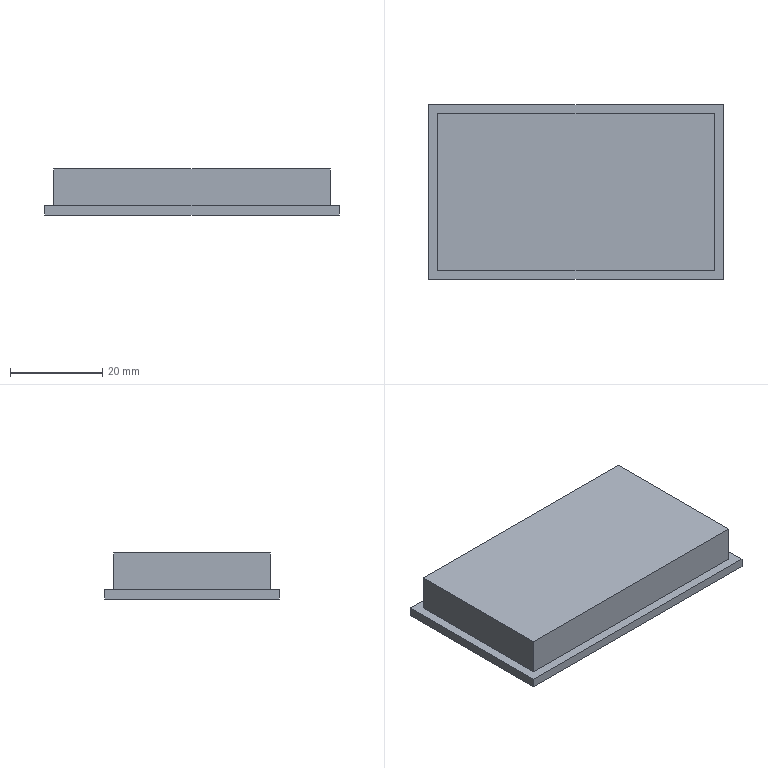Part | SolidWorks | features Extrusion 1, ICE 1 | 1 solid | 11 faces | box 64 x 38 x 10 mm | volume 21184 mm3 | plane 11
STEP:
#1=CARTESIAN_POINT('',(-32.,19.,1.));
#2=VERTEX_POINT('',#1);
#3=CARTESIAN_POINT('',(-32.,-19.,1.));
#4=VERTEX_POINT('',#3);
#5=CARTESIAN_POINT('',(-32.,19.,1.));
#6=DIRECTION('',(0.,-1.,0.));
#7=VECTOR('',#6,1000.);
#8=LINE('',#5,#7);
#9=EDGE_CURVE('',#2,#4,#8,.T.);
#10=ORIENTED_EDGE('',*,*,#9,.T.);
#11=CARTESIAN_POINT('',(32.,-19.,1.));
#12=VERTEX_POINT('',#11);
#13=CARTESIAN_POINT('',(-32.,-19.,1.));
#14=DIRECTION('',(1.,0.,0.));
#15=VECTOR('',#14,1000.);
#16=LINE('',#13,#15);
#17=EDGE_CURVE('',#4,#12,#16,.T.);
#18=ORIENTED_EDGE('',*,*,#17,.T.);
#19=CARTESIAN_POINT('',(32.,19.,1.));
#20=VERTEX_POINT('',#19);
#21=CARTESIAN_POINT('',(32.,-19.,1.));
#22=DIRECTION('',(0.,1.,0.));
#23=VECTOR('',#22,1000.);
#24=LINE('',#21,#23);
#25=EDGE_CURVE('',#12,#20,#24,.T.);
#26=ORIENTED_EDGE('',*,*,#25,.T.);
#27=CARTESIAN_POINT('',(32.,19.,1.));
#28=DIRECTION('',(-1.,0.,0.));
#29=VECTOR('',#28,1000.);
#30=LINE('',#27,#29);
#31=EDGE_CURVE('',#20,#2,#30,.T.);
#32=ORIENTED_EDGE('',*,*,#31,.T.);
#33=EDGE_LOOP('',(#10,#18,#26,#32));
#34=FACE_OUTER_BOUND('',#33,.T.);
#35=CARTESIAN_POINT('',(30.,-17.,1.));
#36=VERTEX_POINT('',#35);
#37=CARTESIAN_POINT('',(-30.,-17.,1.));
#38=VERTEX_POINT('',#37);
#39=CARTESIAN_POINT('',(0.,-17.,1.));
#40=DIRECTION('',(-1.,0.,0.));
#41=VECTOR('',#40,1000.);
#42=LINE('',#39,#41);
#43=EDGE_CURVE('',#36,#38,#42,.T.);
#44=ORIENTED_EDGE('',*,*,#43,.T.);
#45=CARTESIAN_POINT('',(-30.,17.,1.));
#46=VERTEX_POINT('',#45);
#47=CARTESIAN_POINT('',(-30.,0.,1.));
#48=DIRECTION('',(0.,1.,0.));
#49=VECTOR('',#48,1000.);
#50=LINE('',#47,#49);
#51=EDGE_CURVE('',#38,#46,#50,.T.);
#52=ORIENTED_EDGE('',*,*,#51,.T.);
#53=CARTESIAN_POINT('',(30.,17.,1.));
#54=VERTEX_POINT('',#53);
#55=CARTESIAN_POINT('',(0.,17.,1.));
#56=DIRECTION('',(1.,0.,0.));
#57=VECTOR('',#56,1000.);
#58=LINE('',#55,#57);
#59=EDGE_CURVE('',#46,#54,#58,.T.);
#60=ORIENTED_EDGE('',*,*,#59,.T.);
#61=CARTESIAN_POINT('',(30.,0.,1.));
#62=DIRECTION('',(0.,-1.,0.));
#63=VECTOR('',#62,1000.);
#64=LINE('',#61,#63);
#65=EDGE_CURVE('',#54,#36,#64,.T.);
#66=ORIENTED_EDGE('',*,*,#65,.T.);
#67=EDGE_LOOP('',(#44,#52,#60,#66));
#68=FACE_BOUND('',#67,.T.);
#69=CARTESIAN_POINT('',(0.,0.,1.));
#70=DIRECTION('',(0.,0.,1.));
#71=DIRECTION('',(1.,0.,0.));
#72=AXIS2_PLACEMENT_3D('',#69,#70,#71);
#73=PLANE('',#72);
#74=ADVANCED_FACE('',(#34,#68),#73,.T.);
#75=ORIENTED_EDGE('',*,*,#9,.F.);
#76=CARTESIAN_POINT('',(-32.,19.,-1.));
#77=VERTEX_POINT('',#76);
#78=CARTESIAN_POINT('',(-32.,19.,-1.));
#79=DIRECTION('',(0.,0.,1.));
#80=VECTOR('',#79,1000.);
#81=LINE('',#78,#80);
#82=EDGE_CURVE('',#77,#2,#81,.T.);
#83=ORIENTED_EDGE('',*,*,#82,.F.);
#84=CARTESIAN_POINT('',(-32.,-19.,-1.));
#85=VERTEX_POINT('',#84);
#86=CARTESIAN_POINT('',(-32.,19.,-1.));
#87=DIRECTION('',(0.,-1.,0.));
#88=VECTOR('',#87,1000.);
#89=LINE('',#86,#88);
#90=EDGE_CURVE('',#77,#85,#89,.T.);
#91=ORIENTED_EDGE('',*,*,#90,.T.);
#92=CARTESIAN_POINT('',(-32.,-19.,-1.));
#93=DIRECTION('',(0.,0.,1.));
#94=VECTOR('',#93,1000.);
#95=LINE('',#92,#94);
#96=EDGE_CURVE('',#85,#4,#95,.T.);
#97=ORIENTED_EDGE('',*,*,#96,.T.);
#98=EDGE_LOOP('',(#75,#83,#91,#97));
#99=FACE_OUTER_BOUND('',#98,.T.);
#100=CARTESIAN_POINT('',(-32.,19.,-1.));
#101=DIRECTION('',(-1.,0.,0.));
#102=DIRECTION('',(0.,0.,1.));
#103=AXIS2_PLACEMENT_3D('',#100,#101,#102);
#104=PLANE('',#103);
#105=ADVANCED_FACE('',(#99),#104,.T.);
#106=ORIENTED_EDGE('',*,*,#31,.F.);
#107=CARTESIAN_POINT('',(32.,19.,-1.));
#108=VERTEX_POINT('',#107);
#109=CARTESIAN_POINT('',(32.,19.,-1.));
#110=DIRECTION('',(0.,0.,1.));
#111=VECTOR('',#110,1000.);
#112=LINE('',#109,#111);
#113=EDGE_CURVE('',#108,#20,#112,.T.);
#114=ORIENTED_EDGE('',*,*,#113,.F.);
#115=CARTESIAN_POINT('',(32.,19.,-1.));
#116=DIRECTION('',(-1.,0.,0.));
#117=VECTOR('',#116,1000.);
#118=LINE('',#115,#117);
#119=EDGE_CURVE('',#108,#77,#118,.T.);
#120=ORIENTED_EDGE('',*,*,#119,.T.);
#121=ORIENTED_EDGE('',*,*,#82,.T.);
#122=EDGE_LOOP('',(#106,#114,#120,#121));
#123=FACE_OUTER_BOUND('',#122,.T.);
#124=CARTESIAN_POINT('',(32.,19.,-1.));
#125=DIRECTION('',(0.,1.,0.));
#126=DIRECTION('',(0.,0.,1.));
#127=AXIS2_PLACEMENT_3D('',#124,#125,#126);
#128=PLANE('',#127);
#129=ADVANCED_FACE('',(#123),#128,.T.);
#130=ORIENTED_EDGE('',*,*,#25,.F.);
#131=CARTESIAN_POINT('',(32.,-19.,-1.));
#132=VERTEX_POINT('',#131);
#133=CARTESIAN_POINT('',(32.,-19.,-1.));
#134=DIRECTION('',(0.,0.,1.));
#135=VECTOR('',#134,1000.);
#136=LINE('',#133,#135);
#137=EDGE_CURVE('',#132,#12,#136,.T.);
#138=ORIENTED_EDGE('',*,*,#137,.F.);
#139=CARTESIAN_POINT('',(32.,-19.,-1.));
#140=DIRECTION('',(0.,1.,0.));
#141=VECTOR('',#140,1000.);
#142=LINE('',#139,#141);
#143=EDGE_CURVE('',#132,#108,#142,.T.);
#144=ORIENTED_EDGE('',*,*,#143,.T.);
#145=ORIENTED_EDGE('',*,*,#113,.T.);
#146=EDGE_LOOP('',(#130,#138,#144,#145));
#147=FACE_OUTER_BOUND('',#146,.T.);
#148=CARTESIAN_POINT('',(32.,-19.,-1.));
#149=DIRECTION('',(1.,0.,0.));
#150=DIRECTION('',(0.,0.,-1.));
#151=AXIS2_PLACEMENT_3D('',#148,#149,#150);
#152=PLANE('',#151);
#153=ADVANCED_FACE('',(#147),#152,.T.);
#154=ORIENTED_EDGE('',*,*,#17,.F.);
#155=ORIENTED_EDGE('',*,*,#96,.F.);
#156=CARTESIAN_POINT('',(-32.,-19.,-1.));
#157=DIRECTION('',(1.,0.,0.));
#158=VECTOR('',#157,1000.);
#159=LINE('',#156,#158);
#160=EDGE_CURVE('',#85,#132,#159,.T.);
#161=ORIENTED_EDGE('',*,*,#160,.T.);
#162=ORIENTED_EDGE('',*,*,#137,.T.);
#163=EDGE_LOOP('',(#154,#155,#161,#162));
#164=FACE_OUTER_BOUND('',#163,.T.);
#165=CARTESIAN_POINT('',(-32.,-19.,-1.));
#166=DIRECTION('',(0.,-1.,0.));
#167=DIRECTION('',(0.,0.,-1.));
#168=AXIS2_PLACEMENT_3D('',#165,#166,#167);
#169=PLANE('',#168);
#170=ADVANCED_FACE('',(#164),#169,.T.);
#171=ORIENTED_EDGE('',*,*,#90,.F.);
#172=ORIENTED_EDGE('',*,*,#119,.F.);
#173=ORIENTED_EDGE('',*,*,#143,.F.);
#174=ORIENTED_EDGE('',*,*,#160,.F.);
#175=EDGE_LOOP('',(#171,#172,#173,#174));
#176=FACE_OUTER_BOUND('',#175,.T.);
#177=CARTESIAN_POINT('',(0.,0.,-1.));
#178=DIRECTION('',(0.,0.,1.));
#179=DIRECTION('',(1.,0.,0.));
#180=AXIS2_PLACEMENT_3D('',#177,#178,#179);
#181=PLANE('',#180);
#182=ADVANCED_FACE('',(#176),#181,.F.);
#183=ORIENTED_EDGE('',*,*,#51,.F.);
#184=CARTESIAN_POINT('',(-30.,-17.,9.));
#185=VERTEX_POINT('',#184);
#186=CARTESIAN_POINT('',(-30.,-17.,9.));
#187=DIRECTION('',(0.,0.,-1.));
#188=VECTOR('',#187,1000.);
#189=LINE('',#186,#188);
#190=EDGE_CURVE('',#185,#38,#189,.T.);
#191=ORIENTED_EDGE('',*,*,#190,.F.);
#192=CARTESIAN_POINT('',(-30.,17.,9.));
#193=VERTEX_POINT('',#192);
#194=CARTESIAN_POINT('',(-30.,17.,9.));
#195=DIRECTION('',(0.,-1.,0.));
#196=VECTOR('',#195,1000.);
#197=LINE('',#194,#196);
#198=EDGE_CURVE('',#193,#185,#197,.T.);
#199=ORIENTED_EDGE('',*,*,#198,.F.);
#200=CARTESIAN_POINT('',(-30.,17.,9.));
#201=DIRECTION('',(0.,0.,-1.));
#202=VECTOR('',#201,1000.);
#203=LINE('',#200,#202);
#204=EDGE_CURVE('',#193,#46,#203,.T.);
#205=ORIENTED_EDGE('',*,*,#204,.T.);
#206=EDGE_LOOP('',(#183,#191,#199,#205));
#207=FACE_OUTER_BOUND('',#206,.T.);
#208=CARTESIAN_POINT('',(-30.,17.,9.));
#209=DIRECTION('',(1.,0.,0.));
#210=DIRECTION('',(0.,0.,-1.));
#211=AXIS2_PLACEMENT_3D('',#208,#209,#210);
#212=PLANE('',#211);
#213=ADVANCED_FACE('',(#207),#212,.F.);
#214=ORIENTED_EDGE('',*,*,#43,.F.);
#215=CARTESIAN_POINT('',(30.,-17.,9.));
#216=VERTEX_POINT('',#215);
#217=CARTESIAN_POINT('',(30.,-17.,9.));
#218=DIRECTION('',(0.,0.,-1.));
#219=VECTOR('',#218,1000.);
#220=LINE('',#217,#219);
#221=EDGE_CURVE('',#216,#36,#220,.T.);
#222=ORIENTED_EDGE('',*,*,#221,.F.);
#223=CARTESIAN_POINT('',(-30.,-17.,9.));
#224=DIRECTION('',(1.,0.,0.));
#225=VECTOR('',#224,1000.);
#226=LINE('',#223,#225);
#227=EDGE_CURVE('',#185,#216,#226,.T.);
#228=ORIENTED_EDGE('',*,*,#227,.F.);
#229=ORIENTED_EDGE('',*,*,#190,.T.);
#230=EDGE_LOOP('',(#214,#222,#228,#229));
#231=FACE_OUTER_BOUND('',#230,.T.);
#232=CARTESIAN_POINT('',(-30.,-17.,9.));
#233=DIRECTION('',(0.,1.,0.));
#234=DIRECTION('',(0.,0.,1.));
#235=AXIS2_PLACEMENT_3D('',#232,#233,#234);
#236=PLANE('',#235);
#237=ADVANCED_FACE('',(#231),#236,.F.);
#238=ORIENTED_EDGE('',*,*,#65,.F.);
#239=CARTESIAN_POINT('',(30.,17.,9.));
#240=VERTEX_POINT('',#239);
#241=CARTESIAN_POINT('',(30.,17.,9.));
#242=DIRECTION('',(0.,0.,-1.));
#243=VECTOR('',#242,1000.);
#244=LINE('',#241,#243);
#245=EDGE_CURVE('',#240,#54,#244,.T.);
#246=ORIENTED_EDGE('',*,*,#245,.F.);
#247=CARTESIAN_POINT('',(30.,-17.,9.));
#248=DIRECTION('',(0.,1.,0.));
#249=VECTOR('',#248,1000.);
#250=LINE('',#247,#249);
#251=EDGE_CURVE('',#216,#240,#250,.T.);
#252=ORIENTED_EDGE('',*,*,#251,.F.);
#253=ORIENTED_EDGE('',*,*,#221,.T.);
#254=EDGE_LOOP('',(#238,#246,#252,#253));
#255=FACE_OUTER_BOUND('',#254,.T.);
#256=CARTESIAN_POINT('',(30.,-17.,9.));
#257=DIRECTION('',(-1.,0.,0.));
#258=DIRECTION('',(0.,0.,1.));
#259=AXIS2_PLACEMENT_3D('',#256,#257,#258);
#260=PLANE('',#259);
#261=ADVANCED_FACE('',(#255),#260,.F.);
#262=ORIENTED_EDGE('',*,*,#59,.F.);
#263=ORIENTED_EDGE('',*,*,#204,.F.);
#264=CARTESIAN_POINT('',(30.,17.,9.));
#265=DIRECTION('',(-1.,0.,0.));
#266=VECTOR('',#265,1000.);
#267=LINE('',#264,#266);
#268=EDGE_CURVE('',#240,#193,#267,.T.);
#269=ORIENTED_EDGE('',*,*,#268,.F.);
#270=ORIENTED_EDGE('',*,*,#245,.T.);
#271=EDGE_LOOP('',(#262,#263,#269,#270));
#272=FACE_OUTER_BOUND('',#271,.T.);
#273=CARTESIAN_POINT('',(30.,17.,9.));
#274=DIRECTION('',(0.,-1.,0.));
#275=DIRECTION('',(0.,0.,-1.));
#276=AXIS2_PLACEMENT_3D('',#273,#274,#275);
#277=PLANE('',#276);
#278=ADVANCED_FACE('',(#272),#277,.F.);
#279=ORIENTED_EDGE('',*,*,#198,.T.);
#280=ORIENTED_EDGE('',*,*,#227,.T.);
#281=ORIENTED_EDGE('',*,*,#251,.T.);
#282=ORIENTED_EDGE('',*,*,#268,.T.);
#283=EDGE_LOOP('',(#279,#280,#281,#282));
#284=FACE_OUTER_BOUND('',#283,.T.);
#285=CARTESIAN_POINT('',(0.,0.,9.));
#286=DIRECTION('',(0.,0.,1.));
#287=DIRECTION('',(1.,0.,0.));
#288=AXIS2_PLACEMENT_3D('',#285,#286,#287);
#289=PLANE('',#288);
#290=ADVANCED_FACE('',(#284),#289,.T.);
#291=CLOSED_SHELL('',(#74,#105,#129,#153,#170,#182,#213,#237,#261,#278,#290));
#292=MANIFOLD_SOLID_BREP('',#291);
#293=CARTESIAN_POINT('',(0.,0.,0.));
#294=DIRECTION('',(0.,0.,1.));
#295=DIRECTION('',(1.,0.,0.));
#296=AXIS2_PLACEMENT_3D('',#293,#294,#295);
#297=(LENGTH_UNIT()NAMED_UNIT(*)SI_UNIT(.MILLI.,.METRE.));
#298=UNCERTAINTY_MEASURE_WITH_UNIT(LENGTH_MEASURE(0.00001),#297,'','');
#299=(NAMED_UNIT(*)PLANE_ANGLE_UNIT()SI_UNIT($,.RADIAN.));
#300=(NAMED_UNIT(*)SI_UNIT($,.STERADIAN.)SOLID_ANGLE_UNIT());
#301=(GEOMETRIC_REPRESENTATION_CONTEXT(3)GLOBAL_UNCERTAINTY_ASSIGNED_CONTEXT((#298))GLOBAL_UNIT_ASSIGNED_CONTEXT((#297,#299,#300))REPRESENTATION_CONTEXT('',''));
#302=ADVANCED_BREP_SHAPE_REPRESENTATION('',(#292,#296),#301);